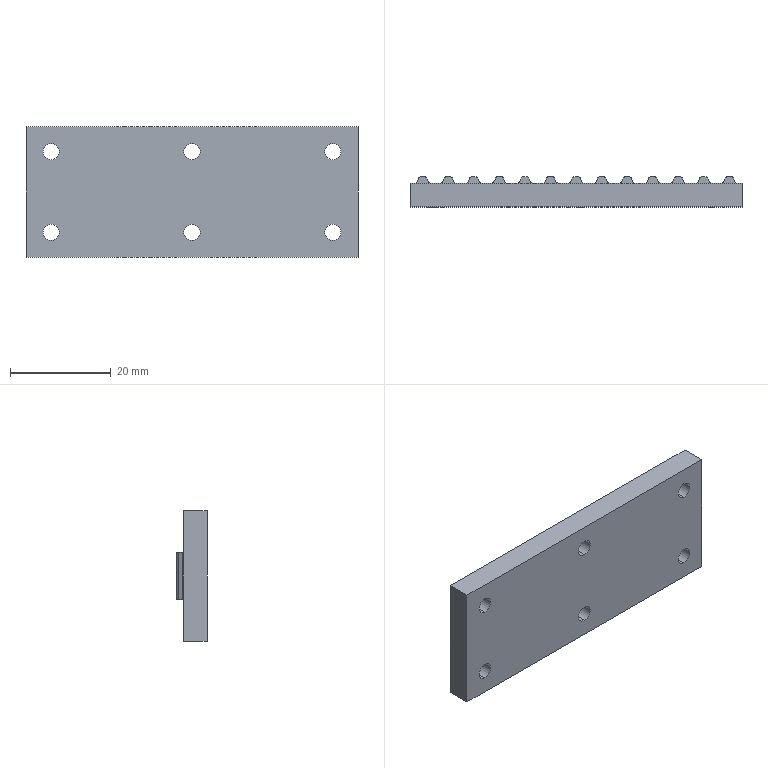Part | SolidWorks | features BaseBody 1 | 1 solid | 135 faces | box 66 x 6 x 26 mm | volume 8148 mm3 | plane 71 | cylinder 64 | commonest cylinder face diameters 0.76 x52 3.242 x12